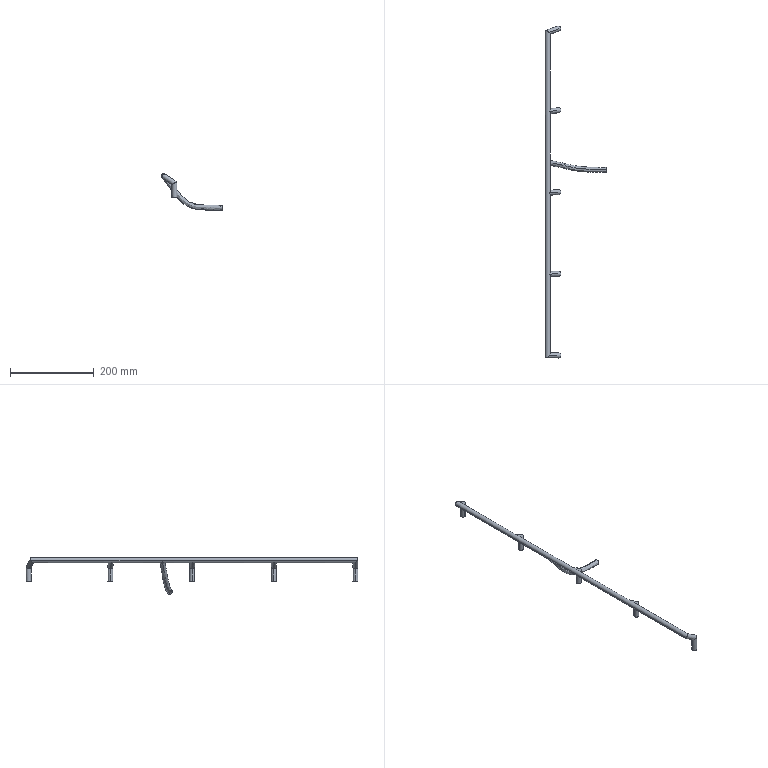Part | SolidWorks | features Sweep 5, 3DProfileFeature 2 | 1 solid | 93 faces | box 146.397 x 792 x 87.372 mm | volume 78940 mm3 | cylinder 71 | plane 14 | spline 8 | commonest cylinder face diameters 8 x36 12 x35